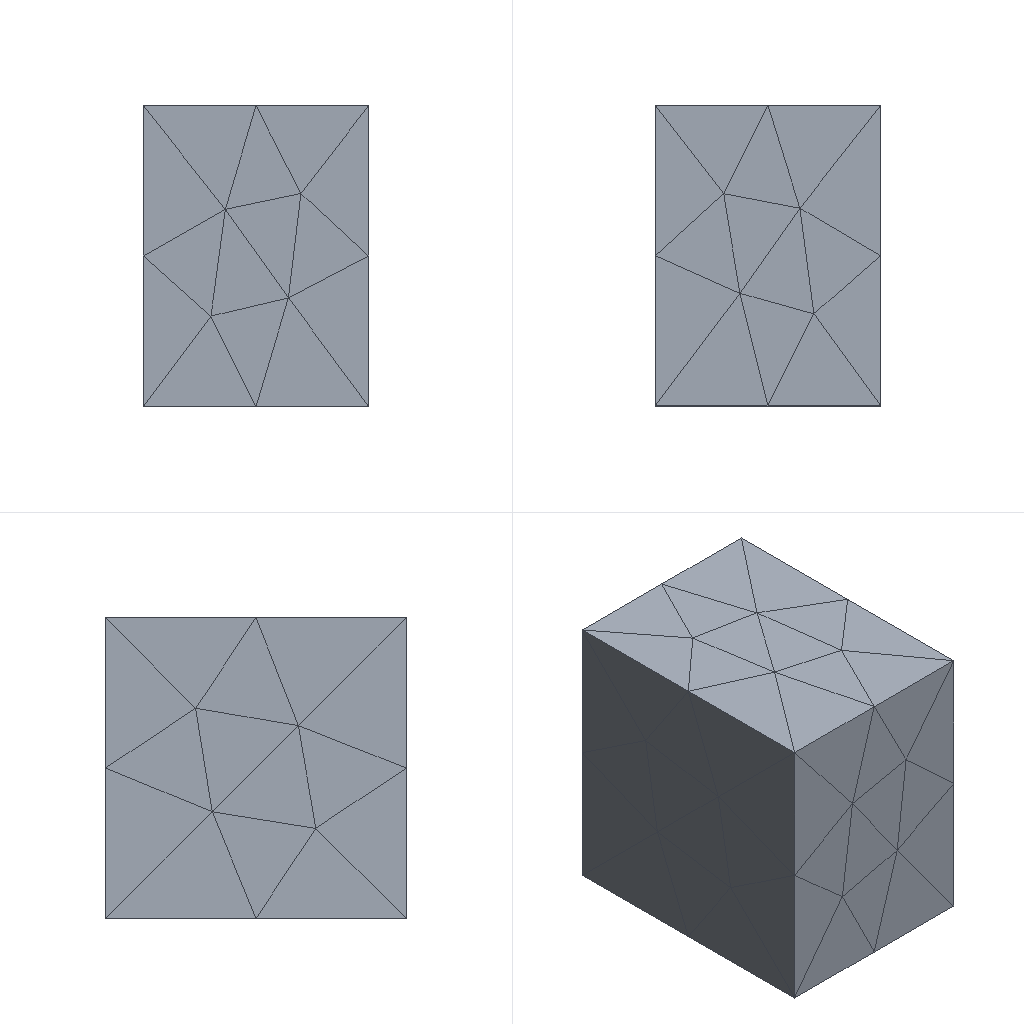Simulation study | ansys mapdl
Set-up summary:
category,name,step,type,value,unit,region
solver,ansys_mapdl
units,mm-N-s-tonne (MPa),,inferred,E=210000 density=
analysis,model,,static
mesh,nodes,,,231
mesh,elements,,,100
element_type,SOLID187,,,100
material,mat 1,,E,210000
material,mat 1,,nu,0.3
load,,model,body load temp,,,all
load,,model,force,"1000 [dir=(0, 0, -1) n=69]",,node list
bc,,model,fixed,"[dofs=UX,UY,UZ n=326]",,node list
Ansys APDL input file, long lists of numbers shortened:
/COM,ANSYS RELEASE 2026 R1           BUILD 26.1      UP20260202       09:08:28
/PREP7
/NOPR
/TITLE,2
ANTYPE, 0
*IF,_CDRDOFF,EQ,1,THEN     !if solid model was read in
_CDRDOFF=             !reset flag, numoffs already performed
*ELSE              !offset database for the following FE model
NUMOFF,NODE,      231
NUMOFF,ELEM,      100
NUMOFF,MAT ,        1
NUMOFF,TYPE,        1
*ENDIF
*SET,_RETURN ,  0.
*SET,_STATUS ,  0.
*SET,_UIQR   ,  69.
*SET,__FLOATPARAMETER__,  231.
DOF,DELETE
ETBLOCK,        1,        1
(2i9,19a9)
        1      187        0        0        0        0        0        0        0        0        0        0        0        0        0        0        0        0        0        0        0
       -1
NBLOCK,6,SOLID,       231,       231
(3i9,6e21.13e3)
        1        0        0 4.1000000000000E+001 8.0000000000000E+000
! (230 more lines like these left out)
N,UNBL,LOC,       -1,
EBLOCK,19,SOLID,       100,       100
(19i10)
         1         1         1         1         0         0         0         0        10         0         1       169       170        73        45       152       172       173       159
! (199 more lines like these left out)
        -1
MPTEMP,UNBL, 1, 1,  0.    ,
MPDATA,UNBL, 1,EX  ,       1, 1,  210000.000    ,
MPTEMP,UNBL, 1, 1,  0.    ,
MPDATA,UNBL, 1,NUXY,       1, 1, 0.3    ,
MPTEMP,UNBL, 1, 1,  0.    ,
MPDATA,UNBL, 1,PRXY,       1, 1, 0.3    ,
EXTOPT,ATTR,      0,      0,      0
EXTOPT,ESIZE,  0,  0.
EXTOPT,ACLEAR,      0
TREF,  0.
IRLF,  0
BFUNIF,TEMP,_TINY
ACEL,  0.    ,  0.    ,  0.
OMEGA,  0.    ,  0.    ,  0.
DOMEGA,  0.    ,  0.    ,  0.
CGLOC,  0.    ,  0.    ,  0.
CGOMEGA,  0.    ,  0.    ,  0.
DCGOMG,  0.    ,  0.    ,  0.
KUSE,     0
TIME,  0.
ALPHAD,  0.
BETAD,  0.
DMPRAT,  0.
DMPSTR,  0.
CRPLIM, 0.1    ,   0
CRPLIM,  0.    ,   1
NCNV,     0, 1.000000000E+12,     0,  0.    ,  0.
NEQIT,     0
ERESX,DEFA
DBLOCK,       326
(i9,a6,2(pg16.9))
        1  UX    0.00000000      0.00000000
! (325 more lines like these left out)
       -1
FBLOCK,        69
(i9,a6,2(pg16.9))
       38  FZ   -14.4927536      0.00000000
! (68 more lines like these left out)
       -1
/GO
FINISH
Results summary:
result,analysis_type_db,,,static,unstated
result,n_sets,,,1,unstated
result,load_steps[0].set,load_step=1,,1,unstated
result,load_steps[0].substep,load_step=1,,1,unstated
result,load_steps[0].time,load_step=1,,1,unstated
result,load_steps[0].freq,load_step=1,,1,unstated
result,load_steps[0].max_usum,load_step=1,,0.0004842,unstated
result,load_steps[0].max_seqv,load_step=1,,9.969,unstated
result,load_steps[0].reaction_sum.FX,load_step=1,,5.20961e-12,unstated
result,load_steps[0].reaction_sum.FY,load_step=1,,2.36469e-11,unstated
result,load_steps[0].reaction_sum.FZ,load_step=1,,1000,unstated
result,load_steps[0].reaction_sum.MX,load_step=1,,0,unstated
result,load_steps[0].reaction_sum.MY,load_step=1,,0,unstated
result,load_steps[0].reaction_sum.MZ,load_step=1,,0,unstated
result,convergence,,,results present for all listed sets,unstated